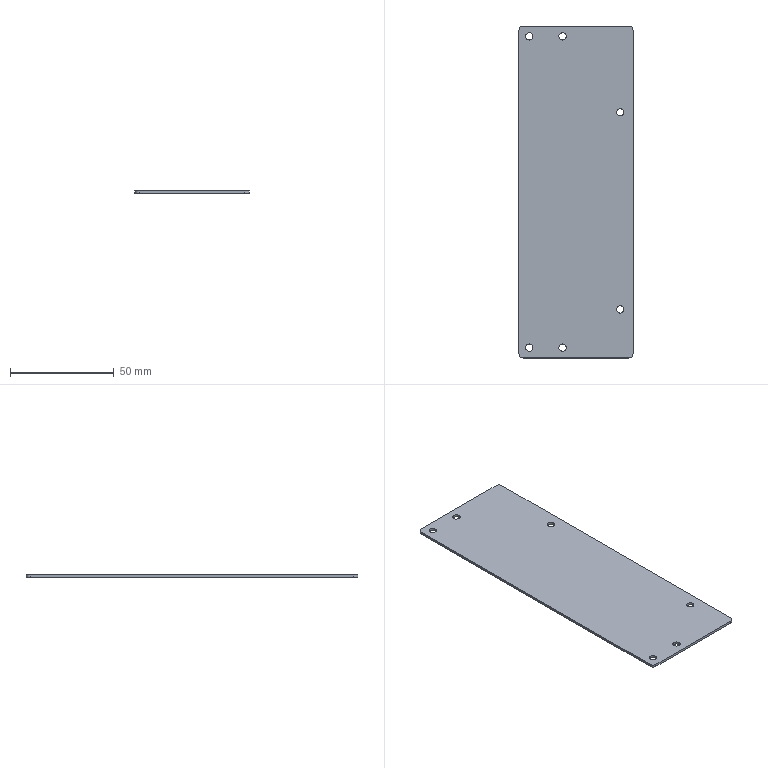Part | STEP file | Mounting block | 1 solid | 16 faces | box 55 x 160 x 1.2 mm | volume 10487 mm3 | cylinder 10 | plane 6 | commonest cylinder face diameters 3.5 x6 4 x4
STEP:
#1=CARTESIAN_POINT('',(0.,0.,0.));
#2=DIRECTION('',(0.,0.,1.));
#3=DIRECTION('',(1.,0.,0.));
#4=AXIS2_PLACEMENT_3D('',#1,#2,#3);
#5=CARTESIAN_POINT('',(-30.,-73.25,1.2));
#6=VERTEX_POINT('',#5);
#7=CARTESIAN_POINT('',(-28.25,-75.,1.2));
#8=VERTEX_POINT('',#7);
#9=CARTESIAN_POINT('',(-30.,-75.,1.2));
#10=DIRECTION('',(0.,0.,-1.));
#11=DIRECTION('',(0.,1.,0.));
#12=AXIS2_PLACEMENT_3D('',#9,#10,#11);
#13=CIRCLE('',#12,1.75);
#14=CARTESIAN_POINT('',(-33.,-78.,1.2));
#15=DIRECTION('',(0.,0.,1.));
#16=DIRECTION('',(1.,0.,0.));
#17=AXIS2_PLACEMENT_3D('',#14,#15,#16);
#18=PLANE('',#17);
#19=CARTESIAN_POINT('',(3.,4.75));
#20=CARTESIAN_POINT('',(6.031,4.75));
#21=CARTESIAN_POINT('',(4.516,2.125));
#22=CARTESIAN_POINT('',(3.,-0.5));
#23=CARTESIAN_POINT('',(1.484,2.125));
#24=CARTESIAN_POINT('',(-0.03109,4.75));
#25=CARTESIAN_POINT('',(3.,4.75));
#26=(BOUNDED_CURVE()B_SPLINE_CURVE(2,(#19,#20,#21,#22,#23,#24,#25),.UNSPECIFIED.,.T.,.F.)B_SPLINE_CURVE_WITH_KNOTS((1,2,2,2,2,1),(-2.094,0.,2.094,4.189,6.283,8.378),.UNSPECIFIED.)CURVE()GEOMETRIC_REPRESENTATION_ITEM()RATIONAL_B_SPLINE_CURVE((1.,0.5,1.,0.5,1.,0.5,1.))REPRESENTATION_ITEM(''));
#27=(GEOMETRIC_REPRESENTATION_CONTEXT(2)PARAMETRIC_REPRESENTATION_CONTEXT()REPRESENTATION_CONTEXT('',''));
#28=DEFINITIONAL_REPRESENTATION('',(#26),#27);
#29=PCURVE('',#18,#28);
#30=CARTESIAN_POINT('',(-30.,-75.,-0.3));
#31=DIRECTION('',(0.,0.,1.));
#32=DIRECTION('',(1.,0.,0.));
#33=AXIS2_PLACEMENT_3D('',#30,#31,#32);
#34=CYLINDRICAL_SURFACE('',#33,1.75);
#35=CARTESIAN_POINT('',(1.571,1.5));
#36=DIRECTION('',(-1.,0.));
#37=VECTOR('',#36,1.);
#38=LINE('',#35,#37);
#39=(GEOMETRIC_REPRESENTATION_CONTEXT(2)PARAMETRIC_REPRESENTATION_CONTEXT()REPRESENTATION_CONTEXT('',''));
#40=DEFINITIONAL_REPRESENTATION('',(#38),#39);
#41=PCURVE('',#34,#40);
#42=SURFACE_CURVE('',#13,(#29,#41),.PCURVE_S1.);
#43=EDGE_CURVE('',#6,#8,#42,.T.);
#44=ORIENTED_EDGE('',*,*,#43,.T.);
#45=CARTESIAN_POINT('',(-30.,-75.,1.2));
#46=DIRECTION('',(0.,0.,-1.));
#47=DIRECTION('',(0.,1.,0.));
#48=AXIS2_PLACEMENT_3D('',#45,#46,#47);
#49=CIRCLE('',#48,1.75);
#50=CARTESIAN_POINT('',(3.,4.75));
#51=CARTESIAN_POINT('',(6.031,4.75));
#52=CARTESIAN_POINT('',(4.516,2.125));
#53=CARTESIAN_POINT('',(3.,-0.5));
#54=CARTESIAN_POINT('',(1.484,2.125));
#55=CARTESIAN_POINT('',(-0.03109,4.75));
#56=CARTESIAN_POINT('',(3.,4.75));
#57=(BOUNDED_CURVE()B_SPLINE_CURVE(2,(#50,#51,#52,#53,#54,#55,#56),.UNSPECIFIED.,.T.,.F.)B_SPLINE_CURVE_WITH_KNOTS((1,2,2,2,2,1),(-2.094,0.,2.094,4.189,6.283,8.378),.UNSPECIFIED.)CURVE()GEOMETRIC_REPRESENTATION_ITEM()RATIONAL_B_SPLINE_CURVE((1.,0.5,1.,0.5,1.,0.5,1.))REPRESENTATION_ITEM(''));
#58=(GEOMETRIC_REPRESENTATION_CONTEXT(2)PARAMETRIC_REPRESENTATION_CONTEXT()REPRESENTATION_CONTEXT('',''));
#59=DEFINITIONAL_REPRESENTATION('',(#57),#58);
#60=PCURVE('',#18,#59);
#61=CARTESIAN_POINT('',(7.854,1.5));
#62=DIRECTION('',(-1.,0.));
#63=VECTOR('',#62,1.);
#64=LINE('',#61,#63);
#65=(GEOMETRIC_REPRESENTATION_CONTEXT(2)PARAMETRIC_REPRESENTATION_CONTEXT()REPRESENTATION_CONTEXT('',''));
#66=DEFINITIONAL_REPRESENTATION('',(#64),#65);
#67=PCURVE('',#34,#66);
#68=SURFACE_CURVE('',#49,(#60,#67),.PCURVE_S1.);
#69=EDGE_CURVE('',#8,#6,#68,.T.);
#70=ORIENTED_EDGE('',*,*,#69,.T.);
#71=EDGE_LOOP('',(#44,#70));
#72=FACE_BOUND('',#71,.T.);
#73=CARTESIAN_POINT('',(-14.,73.25,1.2));
#74=VERTEX_POINT('',#73);
#75=CARTESIAN_POINT('',(-12.25,75.,1.2));
#76=VERTEX_POINT('',#75);
#77=CARTESIAN_POINT('',(-14.,75.,1.2));
#78=DIRECTION('',(0.,0.,1.));
#79=DIRECTION('',(0.,-1.,0.));
#80=AXIS2_PLACEMENT_3D('',#77,#78,#79);
#81=CIRCLE('',#80,1.75);
#82=CARTESIAN_POINT('',(19.,153.));
#83=DIRECTION('',(0.,-1.));
#84=AXIS2_PLACEMENT_2D('',#82,#83);
#85=CIRCLE('',#84,1.75);
#86=(GEOMETRIC_REPRESENTATION_CONTEXT(2)PARAMETRIC_REPRESENTATION_CONTEXT()REPRESENTATION_CONTEXT('',''));
#87=DEFINITIONAL_REPRESENTATION('',(#85),#86);
#88=PCURVE('',#18,#87);
#89=CARTESIAN_POINT('',(-14.,75.,-0.3));
#90=DIRECTION('',(0.,0.,1.));
#91=DIRECTION('',(1.,0.,0.));
#92=AXIS2_PLACEMENT_3D('',#89,#90,#91);
#93=CYLINDRICAL_SURFACE('',#92,1.75);
#94=CARTESIAN_POINT('',(4.712,1.5));
#95=DIRECTION('',(1.,0.));
#96=VECTOR('',#95,1.);
#97=LINE('',#94,#96);
#98=(GEOMETRIC_REPRESENTATION_CONTEXT(2)PARAMETRIC_REPRESENTATION_CONTEXT()REPRESENTATION_CONTEXT('',''));
#99=DEFINITIONAL_REPRESENTATION('',(#97),#98);
#100=PCURVE('',#93,#99);
#101=SURFACE_CURVE('',#81,(#88,#100),.PCURVE_S1.);
#102=EDGE_CURVE('',#74,#76,#101,.T.);
#103=ORIENTED_EDGE('',*,*,#102,.F.);
#104=CARTESIAN_POINT('',(-14.,75.,1.2));
#105=DIRECTION('',(0.,0.,1.));
#106=DIRECTION('',(0.,-1.,0.));
#107=AXIS2_PLACEMENT_3D('',#104,#105,#106);
#108=CIRCLE('',#107,1.75);
#109=CARTESIAN_POINT('',(19.,153.));
#110=DIRECTION('',(0.,-1.));
#111=AXIS2_PLACEMENT_2D('',#109,#110);
#112=CIRCLE('',#111,1.75);
#113=(GEOMETRIC_REPRESENTATION_CONTEXT(2)PARAMETRIC_REPRESENTATION_CONTEXT()REPRESENTATION_CONTEXT('',''));
#114=DEFINITIONAL_REPRESENTATION('',(#112),#113);
#115=PCURVE('',#18,#114);
#116=CARTESIAN_POINT('',(-1.571,1.5));
#117=DIRECTION('',(1.,0.));
#118=VECTOR('',#117,1.);
#119=LINE('',#116,#118);
#120=(GEOMETRIC_REPRESENTATION_CONTEXT(2)PARAMETRIC_REPRESENTATION_CONTEXT()REPRESENTATION_CONTEXT('',''));
#121=DEFINITIONAL_REPRESENTATION('',(#119),#120);
#122=PCURVE('',#93,#121);
#123=SURFACE_CURVE('',#108,(#115,#122),.PCURVE_S1.);
#124=EDGE_CURVE('',#76,#74,#123,.T.);
#125=ORIENTED_EDGE('',*,*,#124,.F.);
#126=EDGE_LOOP('',(#103,#125));
#127=FACE_BOUND('',#126,.T.);
#128=CARTESIAN_POINT('',(15.595,-56.595,1.2));
#129=VERTEX_POINT('',#128);
#130=CARTESIAN_POINT('',(13.845,-54.845,1.2));
#131=VERTEX_POINT('',#130);
#132=CARTESIAN_POINT('',(13.845,-56.595,1.2));
#133=DIRECTION('',(0.,0.,1.));
#134=DIRECTION('',(1.,0.,0.));
#135=AXIS2_PLACEMENT_3D('',#132,#133,#134);
#136=CIRCLE('',#135,1.75);
#137=CARTESIAN_POINT('',(46.845,21.405));
#138=DIRECTION('',(1.,0.));
#139=AXIS2_PLACEMENT_2D('',#137,#138);
#140=CIRCLE('',#139,1.75);
#141=(GEOMETRIC_REPRESENTATION_CONTEXT(2)PARAMETRIC_REPRESENTATION_CONTEXT()REPRESENTATION_CONTEXT('',''));
#142=DEFINITIONAL_REPRESENTATION('',(#140),#141);
#143=PCURVE('',#18,#142);
#144=CARTESIAN_POINT('',(13.845,-56.595,1.5));
#145=DIRECTION('',(0.,0.,-1.));
#146=DIRECTION('',(-1.,0.,0.));
#147=AXIS2_PLACEMENT_3D('',#144,#145,#146);
#148=CYLINDRICAL_SURFACE('',#147,1.75);
#149=CARTESIAN_POINT('',(3.142,0.3));
#150=DIRECTION('',(-1.,0.));
#151=VECTOR('',#150,1.);
#152=LINE('',#149,#151);
#153=(GEOMETRIC_REPRESENTATION_CONTEXT(2)PARAMETRIC_REPRESENTATION_CONTEXT()REPRESENTATION_CONTEXT('',''));
#154=DEFINITIONAL_REPRESENTATION('',(#152),#153);
#155=PCURVE('',#148,#154);
#156=SURFACE_CURVE('',#136,(#143,#155),.PCURVE_S1.);
#157=EDGE_CURVE('',#129,#131,#156,.T.);
#158=ORIENTED_EDGE('',*,*,#157,.F.);
#159=CARTESIAN_POINT('',(13.845,-56.595,1.2));
#160=DIRECTION('',(0.,0.,1.));
#161=DIRECTION('',(1.,0.,0.));
#162=AXIS2_PLACEMENT_3D('',#159,#160,#161);
#163=CIRCLE('',#162,1.75);
#164=CARTESIAN_POINT('',(46.845,21.405));
#165=DIRECTION('',(1.,0.));
#166=AXIS2_PLACEMENT_2D('',#164,#165);
#167=CIRCLE('',#166,1.75);
#168=(GEOMETRIC_REPRESENTATION_CONTEXT(2)PARAMETRIC_REPRESENTATION_CONTEXT()REPRESENTATION_CONTEXT('',''));
#169=DEFINITIONAL_REPRESENTATION('',(#167),#168);
#170=PCURVE('',#18,#169);
#171=CARTESIAN_POINT('',(9.425,0.3));
#172=DIRECTION('',(-1.,0.));
#173=VECTOR('',#172,1.);
#174=LINE('',#171,#173);
#175=(GEOMETRIC_REPRESENTATION_CONTEXT(2)PARAMETRIC_REPRESENTATION_CONTEXT()REPRESENTATION_CONTEXT('',''));
#176=DEFINITIONAL_REPRESENTATION('',(#174),#175);
#177=PCURVE('',#148,#176);
#178=SURFACE_CURVE('',#163,(#170,#177),.PCURVE_S1.);
#179=EDGE_CURVE('',#131,#129,#178,.T.);
#180=ORIENTED_EDGE('',*,*,#179,.F.);
#181=EDGE_LOOP('',(#158,#180));
#182=FACE_BOUND('',#181,.T.);
#183=CARTESIAN_POINT('',(15.595,38.405,1.2));
#184=VERTEX_POINT('',#183);
#185=CARTESIAN_POINT('',(13.845,40.155,1.2));
#186=VERTEX_POINT('',#185);
#187=CARTESIAN_POINT('',(13.845,38.405,1.2));
#188=DIRECTION('',(0.,0.,1.));
#189=DIRECTION('',(1.,0.,0.));
#190=AXIS2_PLACEMENT_3D('',#187,#188,#189);
#191=CIRCLE('',#190,1.75);
#192=CARTESIAN_POINT('',(46.845,116.405));
#193=DIRECTION('',(1.,0.));
#194=AXIS2_PLACEMENT_2D('',#192,#193);
#195=CIRCLE('',#194,1.75);
#196=(GEOMETRIC_REPRESENTATION_CONTEXT(2)PARAMETRIC_REPRESENTATION_CONTEXT()REPRESENTATION_CONTEXT('',''));
#197=DEFINITIONAL_REPRESENTATION('',(#195),#196);
#198=PCURVE('',#18,#197);
#199=CARTESIAN_POINT('',(13.845,38.405,1.5));
#200=DIRECTION('',(0.,0.,-1.));
#201=DIRECTION('',(-1.,0.,0.));
#202=AXIS2_PLACEMENT_3D('',#199,#200,#201);
#203=CYLINDRICAL_SURFACE('',#202,1.75);
#204=CARTESIAN_POINT('',(3.142,0.3));
#205=DIRECTION('',(-1.,0.));
#206=VECTOR('',#205,1.);
#207=LINE('',#204,#206);
#208=(GEOMETRIC_REPRESENTATION_CONTEXT(2)PARAMETRIC_REPRESENTATION_CONTEXT()REPRESENTATION_CONTEXT('',''));
#209=DEFINITIONAL_REPRESENTATION('',(#207),#208);
#210=PCURVE('',#203,#209);
#211=SURFACE_CURVE('',#191,(#198,#210),.PCURVE_S1.);
#212=EDGE_CURVE('',#184,#186,#211,.T.);
#213=ORIENTED_EDGE('',*,*,#212,.F.);
#214=CARTESIAN_POINT('',(13.845,38.405,1.2));
#215=DIRECTION('',(0.,0.,1.));
#216=DIRECTION('',(1.,0.,0.));
#217=AXIS2_PLACEMENT_3D('',#214,#215,#216);
#218=CIRCLE('',#217,1.75);
#219=CARTESIAN_POINT('',(46.845,116.405));
#220=DIRECTION('',(1.,0.));
#221=AXIS2_PLACEMENT_2D('',#219,#220);
#222=CIRCLE('',#221,1.75);
#223=(GEOMETRIC_REPRESENTATION_CONTEXT(2)PARAMETRIC_REPRESENTATION_CONTEXT()REPRESENTATION_CONTEXT('',''));
#224=DEFINITIONAL_REPRESENTATION('',(#222),#223);
#225=PCURVE('',#18,#224);
#226=CARTESIAN_POINT('',(9.425,0.3));
#227=DIRECTION('',(-1.,0.));
#228=VECTOR('',#227,1.);
#229=LINE('',#226,#228);
#230=(GEOMETRIC_REPRESENTATION_CONTEXT(2)PARAMETRIC_REPRESENTATION_CONTEXT()REPRESENTATION_CONTEXT('',''));
#231=DEFINITIONAL_REPRESENTATION('',(#229),#230);
#232=PCURVE('',#203,#231);
#233=SURFACE_CURVE('',#218,(#225,#232),.PCURVE_S1.);
#234=EDGE_CURVE('',#186,#184,#233,.T.);
#235=ORIENTED_EDGE('',*,*,#234,.F.);
#236=EDGE_LOOP('',(#213,#235));
#237=FACE_BOUND('',#236,.T.);
#238=CARTESIAN_POINT('',(-35.,78.,1.2));
#239=VERTEX_POINT('',#238);
#240=CARTESIAN_POINT('',(-35.,-78.,1.2));
#241=VERTEX_POINT('',#240);
#242=CARTESIAN_POINT('',(-35.,78.,1.2));
#243=DIRECTION('',(0.,-1.,0.));
#244=VECTOR('',#243,1.);
#245=LINE('',#242,#244);
#246=CARTESIAN_POINT('',(-2.,156.));
#247=DIRECTION('',(0.,-1.));
#248=VECTOR('',#247,1.);
#249=LINE('',#246,#248);
#250=(GEOMETRIC_REPRESENTATION_CONTEXT(2)PARAMETRIC_REPRESENTATION_CONTEXT()REPRESENTATION_CONTEXT('',''));
#251=DEFINITIONAL_REPRESENTATION('',(#249),#250);
#252=PCURVE('',#18,#251);
#253=CARTESIAN_POINT('',(-35.,78.,1.2));
#254=DIRECTION('',(1.,0.,0.));
#255=DIRECTION('',(0.,1.,0.));
#256=AXIS2_PLACEMENT_3D('',#253,#254,#255);
#257=PLANE('',#256);
#258=CARTESIAN_POINT('',(0.,0.));
#259=DIRECTION('',(-1.,0.));
#260=VECTOR('',#259,1.);
#261=LINE('',#258,#260);
#262=(GEOMETRIC_REPRESENTATION_CONTEXT(2)PARAMETRIC_REPRESENTATION_CONTEXT()REPRESENTATION_CONTEXT('',''));
#263=DEFINITIONAL_REPRESENTATION('',(#261),#262);
#264=PCURVE('',#257,#263);
#265=SURFACE_CURVE('',#245,(#252,#264),.PCURVE_S1.);
#266=EDGE_CURVE('',#239,#241,#265,.T.);
#267=ORIENTED_EDGE('',*,*,#266,.T.);
#268=CARTESIAN_POINT('',(-33.,-80.,1.2));
#269=VERTEX_POINT('',#268);
#270=CARTESIAN_POINT('',(-33.,-78.,1.2));
#271=DIRECTION('',(0.,0.,1.));
#272=DIRECTION('',(1.,0.,0.));
#273=AXIS2_PLACEMENT_3D('',#270,#271,#272);
#274=CIRCLE('',#273,2.);
#275=CARTESIAN_POINT('',(0.,0.));
#276=DIRECTION('',(1.,0.));
#277=AXIS2_PLACEMENT_2D('',#275,#276);
#278=CIRCLE('',#277,2.);
#279=(GEOMETRIC_REPRESENTATION_CONTEXT(2)PARAMETRIC_REPRESENTATION_CONTEXT()REPRESENTATION_CONTEXT('',''));
#280=DEFINITIONAL_REPRESENTATION('',(#278),#279);
#281=PCURVE('',#18,#280);
#282=CARTESIAN_POINT('',(-33.,-78.,1.2));
#283=DIRECTION('',(0.,0.,-1.));
#284=DIRECTION('',(-1.,0.,0.));
#285=AXIS2_PLACEMENT_3D('',#282,#283,#284);
#286=CYLINDRICAL_SURFACE('',#285,2.);
#287=CARTESIAN_POINT('',(9.425,0.));
#288=DIRECTION('',(-1.,0.));
#289=VECTOR('',#288,1.);
#290=LINE('',#287,#289);
#291=(GEOMETRIC_REPRESENTATION_CONTEXT(2)PARAMETRIC_REPRESENTATION_CONTEXT()REPRESENTATION_CONTEXT('',''));
#292=DEFINITIONAL_REPRESENTATION('',(#290),#291);
#293=PCURVE('',#286,#292);
#294=SURFACE_CURVE('',#274,(#281,#293),.PCURVE_S1.);
#295=EDGE_CURVE('',#241,#269,#294,.T.);
#296=ORIENTED_EDGE('',*,*,#295,.T.);
#297=CARTESIAN_POINT('',(18.,-80.,1.2));
#298=VERTEX_POINT('',#297);
#299=CARTESIAN_POINT('',(-33.,-80.,1.2));
#300=DIRECTION('',(1.,0.,0.));
#301=VECTOR('',#300,1.);
#302=LINE('',#299,#301);
#303=CARTESIAN_POINT('',(0.,-2.));
#304=DIRECTION('',(1.,0.));
#305=VECTOR('',#304,1.);
#306=LINE('',#303,#305);
#307=(GEOMETRIC_REPRESENTATION_CONTEXT(2)PARAMETRIC_REPRESENTATION_CONTEXT()REPRESENTATION_CONTEXT('',''));
#308=DEFINITIONAL_REPRESENTATION('',(#306),#307);
#309=PCURVE('',#18,#308);
#310=CARTESIAN_POINT('',(-33.,-80.,1.2));
#311=DIRECTION('',(0.,1.,0.));
#312=DIRECTION('',(0.,0.,1.));
#313=AXIS2_PLACEMENT_3D('',#310,#311,#312);
#314=PLANE('',#313);
#315=CARTESIAN_POINT('',(0.,0.));
#316=DIRECTION('',(0.,1.));
#317=VECTOR('',#316,1.);
#318=LINE('',#315,#317);
#319=(GEOMETRIC_REPRESENTATION_CONTEXT(2)PARAMETRIC_REPRESENTATION_CONTEXT()REPRESENTATION_CONTEXT('',''));
#320=DEFINITIONAL_REPRESENTATION('',(#318),#319);
#321=PCURVE('',#314,#320);
#322=SURFACE_CURVE('',#302,(#309,#321),.PCURVE_S1.);
#323=EDGE_CURVE('',#269,#298,#322,.T.);
#324=ORIENTED_EDGE('',*,*,#323,.T.);
#325=CARTESIAN_POINT('',(20.,-78.,1.2));
#326=VERTEX_POINT('',#325);
#327=CARTESIAN_POINT('',(18.,-78.,1.2));
#328=DIRECTION('',(0.,0.,1.));
#329=DIRECTION('',(1.,0.,0.));
#330=AXIS2_PLACEMENT_3D('',#327,#328,#329);
#331=CIRCLE('',#330,2.);
#332=CARTESIAN_POINT('',(51.,0.));
#333=DIRECTION('',(1.,0.));
#334=AXIS2_PLACEMENT_2D('',#332,#333);
#335=CIRCLE('',#334,2.);
#336=(GEOMETRIC_REPRESENTATION_CONTEXT(2)PARAMETRIC_REPRESENTATION_CONTEXT()REPRESENTATION_CONTEXT('',''));
#337=DEFINITIONAL_REPRESENTATION('',(#335),#336);
#338=PCURVE('',#18,#337);
#339=CARTESIAN_POINT('',(18.,-78.,1.2));
#340=DIRECTION('',(0.,0.,-1.));
#341=DIRECTION('',(-1.,0.,0.));
#342=AXIS2_PLACEMENT_3D('',#339,#340,#341);
#343=CYLINDRICAL_SURFACE('',#342,2.);
#344=CARTESIAN_POINT('',(9.425,0.));
#345=DIRECTION('',(-1.,0.));
#346=VECTOR('',#345,1.);
#347=LINE('',#344,#346);
#348=(GEOMETRIC_REPRESENTATION_CONTEXT(2)PARAMETRIC_REPRESENTATION_CONTEXT()REPRESENTATION_CONTEXT('',''));
#349=DEFINITIONAL_REPRESENTATION('',(#347),#348);
#350=PCURVE('',#343,#349);
#351=SURFACE_CURVE('',#331,(#338,#350),.PCURVE_S1.);
#352=EDGE_CURVE('',#298,#326,#351,.T.);
#353=ORIENTED_EDGE('',*,*,#352,.T.);
#354=CARTESIAN_POINT('',(20.,78.,1.2));
#355=VERTEX_POINT('',#354);
#356=CARTESIAN_POINT('',(20.,-78.,1.2));
#357=DIRECTION('',(0.,1.,0.));
#358=VECTOR('',#357,1.);
#359=LINE('',#356,#358);
#360=CARTESIAN_POINT('',(53.,0.));
#361=DIRECTION('',(0.,1.));
#362=VECTOR('',#361,1.);
#363=LINE('',#360,#362);
#364=(GEOMETRIC_REPRESENTATION_CONTEXT(2)PARAMETRIC_REPRESENTATION_CONTEXT()REPRESENTATION_CONTEXT('',''));
#365=DEFINITIONAL_REPRESENTATION('',(#363),#364);
#366=PCURVE('',#18,#365);
#367=CARTESIAN_POINT('',(20.,-78.,1.2));
#368=DIRECTION('',(-1.,0.,0.));
#369=DIRECTION('',(0.,-1.,0.));
#370=AXIS2_PLACEMENT_3D('',#367,#368,#369);
#371=PLANE('',#370);
#372=CARTESIAN_POINT('',(0.,0.));
#373=DIRECTION('',(-1.,0.));
#374=VECTOR('',#373,1.);
#375=LINE('',#372,#374);
#376=(GEOMETRIC_REPRESENTATION_CONTEXT(2)PARAMETRIC_REPRESENTATION_CONTEXT()REPRESENTATION_CONTEXT('',''));
#377=DEFINITIONAL_REPRESENTATION('',(#375),#376);
#378=PCURVE('',#371,#377);
#379=SURFACE_CURVE('',#359,(#366,#378),.PCURVE_S1.);
#380=EDGE_CURVE('',#326,#355,#379,.T.);
#381=ORIENTED_EDGE('',*,*,#380,.T.);
#382=CARTESIAN_POINT('',(18.,80.,1.2));
#383=VERTEX_POINT('',#382);
#384=CARTESIAN_POINT('',(18.,78.,1.2));
#385=DIRECTION('',(0.,0.,1.));
#386=DIRECTION('',(1.,0.,0.));
#387=AXIS2_PLACEMENT_3D('',#384,#385,#386);
#388=CIRCLE('',#387,2.);
#389=CARTESIAN_POINT('',(51.,156.));
#390=DIRECTION('',(1.,0.));
#391=AXIS2_PLACEMENT_2D('',#389,#390);
#392=CIRCLE('',#391,2.);
#393=(GEOMETRIC_REPRESENTATION_CONTEXT(2)PARAMETRIC_REPRESENTATION_CONTEXT()REPRESENTATION_CONTEXT('',''));
#394=DEFINITIONAL_REPRESENTATION('',(#392),#393);
#395=PCURVE('',#18,#394);
#396=CARTESIAN_POINT('',(18.,78.,1.2));
#397=DIRECTION('',(0.,0.,-1.));
#398=DIRECTION('',(-1.,0.,0.));
#399=AXIS2_PLACEMENT_3D('',#396,#397,#398);
#400=CYLINDRICAL_SURFACE('',#399,2.);
#401=CARTESIAN_POINT('',(3.142,0.));
#402=DIRECTION('',(-1.,0.));
#403=VECTOR('',#402,1.);
#404=LINE('',#401,#403);
#405=(GEOMETRIC_REPRESENTATION_CONTEXT(2)PARAMETRIC_REPRESENTATION_CONTEXT()REPRESENTATION_CONTEXT('',''));
#406=DEFINITIONAL_REPRESENTATION('',(#404),#405);
#407=PCURVE('',#400,#406);
#408=SURFACE_CURVE('',#388,(#395,#407),.PCURVE_S1.);
#409=EDGE_CURVE('',#355,#383,#408,.T.);
#410=ORIENTED_EDGE('',*,*,#409,.T.);
#411=CARTESIAN_POINT('',(-33.,80.,1.2));
#412=VERTEX_POINT('',#411);
#413=CARTESIAN_POINT('',(18.,80.,1.2));
#414=DIRECTION('',(-1.,0.,0.));
#415=VECTOR('',#414,1.);
#416=LINE('',#413,#415);
#417=CARTESIAN_POINT('',(51.,158.));
#418=DIRECTION('',(-1.,0.));
#419=VECTOR('',#418,1.);
#420=LINE('',#417,#419);
#421=(GEOMETRIC_REPRESENTATION_CONTEXT(2)PARAMETRIC_REPRESENTATION_CONTEXT()REPRESENTATION_CONTEXT('',''));
#422=DEFINITIONAL_REPRESENTATION('',(#420),#421);
#423=PCURVE('',#18,#422);
#424=CARTESIAN_POINT('',(18.,80.,1.2));
#425=DIRECTION('',(0.,-1.,0.));
#426=DIRECTION('',(0.,0.,-1.));
#427=AXIS2_PLACEMENT_3D('',#424,#425,#426);
#428=PLANE('',#427);
#429=CARTESIAN_POINT('',(0.,0.));
#430=DIRECTION('',(0.,-1.));
#431=VECTOR('',#430,1.);
#432=LINE('',#429,#431);
#433=(GEOMETRIC_REPRESENTATION_CONTEXT(2)PARAMETRIC_REPRESENTATION_CONTEXT()REPRESENTATION_CONTEXT('',''));
#434=DEFINITIONAL_REPRESENTATION('',(#432),#433);
#435=PCURVE('',#428,#434);
#436=SURFACE_CURVE('',#416,(#423,#435),.PCURVE_S1.);
#437=EDGE_CURVE('',#383,#412,#436,.T.);
#438=ORIENTED_EDGE('',*,*,#437,.T.);
#439=CARTESIAN_POINT('',(-33.,78.,1.2));
#440=DIRECTION('',(0.,0.,1.));
#441=DIRECTION('',(1.,0.,0.));
#442=AXIS2_PLACEMENT_3D('',#439,#440,#441);
#443=CIRCLE('',#442,2.);
#444=CARTESIAN_POINT('',(0.,156.));
#445=DIRECTION('',(1.,0.));
#446=AXIS2_PLACEMENT_2D('',#444,#445);
#447=CIRCLE('',#446,2.);
#448=(GEOMETRIC_REPRESENTATION_CONTEXT(2)PARAMETRIC_REPRESENTATION_CONTEXT()REPRESENTATION_CONTEXT('',''));
#449=DEFINITIONAL_REPRESENTATION('',(#447),#448);
#450=PCURVE('',#18,#449);
#451=CARTESIAN_POINT('',(-33.,78.,1.2));
#452=DIRECTION('',(0.,0.,-1.));
#453=DIRECTION('',(-1.,0.,0.));
#454=AXIS2_PLACEMENT_3D('',#451,#452,#453);
#455=CYLINDRICAL_SURFACE('',#454,2.);
#456=CARTESIAN_POINT('',(3.142,0.));
#457=DIRECTION('',(-1.,0.));
#458=VECTOR('',#457,1.);
#459=LINE('',#456,#458);
#460=(GEOMETRIC_REPRESENTATION_CONTEXT(2)PARAMETRIC_REPRESENTATION_CONTEXT()REPRESENTATION_CONTEXT('',''));
#461=DEFINITIONAL_REPRESENTATION('',(#459),#460);
#462=PCURVE('',#455,#461);
#463=SURFACE_CURVE('',#443,(#450,#462),.PCURVE_S1.);
#464=EDGE_CURVE('',#412,#239,#463,.T.);
#465=ORIENTED_EDGE('',*,*,#464,.T.);
#466=EDGE_LOOP('',(#267,#296,#324,#353,#381,#410,#438,#465));
#467=FACE_BOUND('',#466,.T.);
#468=CARTESIAN_POINT('',(-30.,73.25,1.2));
#469=VERTEX_POINT('',#468);
#470=CARTESIAN_POINT('',(-28.25,75.,1.2));
#471=VERTEX_POINT('',#470);
#472=CARTESIAN_POINT('',(-30.,75.,1.2));
#473=DIRECTION('',(0.,0.,1.));
#474=DIRECTION('',(0.,-1.,0.));
#475=AXIS2_PLACEMENT_3D('',#472,#473,#474);
#476=CIRCLE('',#475,1.75);
#477=CARTESIAN_POINT('',(3.,153.));
#478=DIRECTION('',(0.,-1.));
#479=AXIS2_PLACEMENT_2D('',#477,#478);
#480=CIRCLE('',#479,1.75);
#481=(GEOMETRIC_REPRESENTATION_CONTEXT(2)PARAMETRIC_REPRESENTATION_CONTEXT()REPRESENTATION_CONTEXT('',''));
#482=DEFINITIONAL_REPRESENTATION('',(#480),#481);
#483=PCURVE('',#18,#482);
#484=CARTESIAN_POINT('',(-30.,75.,-0.3));
#485=DIRECTION('',(0.,0.,1.));
#486=DIRECTION('',(1.,0.,0.));
#487=AXIS2_PLACEMENT_3D('',#484,#485,#486);
#488=CYLINDRICAL_SURFACE('',#487,1.75);
#489=CARTESIAN_POINT('',(4.712,1.5));
#490=DIRECTION('',(1.,0.));
#491=VECTOR('',#490,1.);
#492=LINE('',#489,#491);
#493=(GEOMETRIC_REPRESENTATION_CONTEXT(2)PARAMETRIC_REPRESENTATION_CONTEXT()REPRESENTATION_CONTEXT('',''));
#494=DEFINITIONAL_REPRESENTATION('',(#492),#493);
#495=PCURVE('',#488,#494);
#496=SURFACE_CURVE('',#476,(#483,#495),.PCURVE_S1.);
#497=EDGE_CURVE('',#469,#471,#496,.T.);
#498=ORIENTED_EDGE('',*,*,#497,.F.);
#499=CARTESIAN_POINT('',(-30.,75.,1.2));
#500=DIRECTION('',(0.,0.,1.));
#501=DIRECTION('',(0.,-1.,0.));
#502=AXIS2_PLACEMENT_3D('',#499,#500,#501);
#503=CIRCLE('',#502,1.75);
#504=CARTESIAN_POINT('',(3.,153.));
#505=DIRECTION('',(0.,-1.));
#506=AXIS2_PLACEMENT_2D('',#504,#505);
#507=CIRCLE('',#506,1.75);
#508=(GEOMETRIC_REPRESENTATION_CONTEXT(2)PARAMETRIC_REPRESENTATION_CONTEXT()REPRESENTATION_CONTEXT('',''));
#509=DEFINITIONAL_REPRESENTATION('',(#507),#508);
#510=PCURVE('',#18,#509);
#511=CARTESIAN_POINT('',(-1.571,1.5));
#512=DIRECTION('',(1.,0.));
#513=VECTOR('',#512,1.);
#514=LINE('',#511,#513);
#515=(GEOMETRIC_REPRESENTATION_CONTEXT(2)PARAMETRIC_REPRESENTATION_CONTEXT()REPRESENTATION_CONTEXT('',''));
#516=DEFINITIONAL_REPRESENTATION('',(#514),#515);
#517=PCURVE('',#488,#516);
#518=SURFACE_CURVE('',#503,(#510,#517),.PCURVE_S1.);
#519=EDGE_CURVE('',#471,#469,#518,.T.);
#520=ORIENTED_EDGE('',*,*,#519,.F.);
#521=EDGE_LOOP('',(#498,#520));
#522=FACE_BOUND('',#521,.T.);
#523=CARTESIAN_POINT('',(-14.,-73.25,1.2));
#524=VERTEX_POINT('',#523);
#525=CARTESIAN_POINT('',(-12.25,-75.,1.2));
#526=VERTEX_POINT('',#525);
#527=CARTESIAN_POINT('',(-14.,-75.,1.2));
#528=DIRECTION('',(0.,0.,-1.));
#529=DIRECTION('',(0.,1.,0.));
#530=AXIS2_PLACEMENT_3D('',#527,#528,#529);
#531=CIRCLE('',#530,1.75);
#532=CARTESIAN_POINT('',(19.,4.75));
#533=CARTESIAN_POINT('',(22.031,4.75));
#534=CARTESIAN_POINT('',(20.516,2.125));
#535=CARTESIAN_POINT('',(19.,-0.5));
#536=CARTESIAN_POINT('',(17.484,2.125));
#537=CARTESIAN_POINT('',(15.969,4.75));
#538=CARTESIAN_POINT('',(19.,4.75));
#539=(BOUNDED_CURVE()B_SPLINE_CURVE(2,(#532,#533,#534,#535,#536,#537,#538),.UNSPECIFIED.,.T.,.F.)B_SPLINE_CURVE_WITH_KNOTS((1,2,2,2,2,1),(-2.094,0.,2.094,4.189,6.283,8.378),.UNSPECIFIED.)CURVE()GEOMETRIC_REPRESENTATION_ITEM()RATIONAL_B_SPLINE_CURVE((1.,0.5,1.,0.5,1.,0.5,1.))REPRESENTATION_ITEM(''));
#540=(GEOMETRIC_REPRESENTATION_CONTEXT(2)PARAMETRIC_REPRESENTATION_CONTEXT()REPRESENTATION_CONTEXT('',''));
#541=DEFINITIONAL_REPRESENTATION('',(#539),#540);
#542=PCURVE('',#18,#541);
#543=CARTESIAN_POINT('',(-14.,-75.,-0.3));
#544=DIRECTION('',(0.,0.,1.));
#545=DIRECTION('',(1.,0.,0.));
#546=AXIS2_PLACEMENT_3D('',#543,#544,#545);
#547=CYLINDRICAL_SURFACE('',#546,1.75);
#548=CARTESIAN_POINT('',(1.571,1.5));
#549=DIRECTION('',(-1.,0.));
#550=VECTOR('',#549,1.);
#551=LINE('',#548,#550);
#552=(GEOMETRIC_REPRESENTATION_CONTEXT(2)PARAMETRIC_REPRESENTATION_CONTEXT()REPRESENTATION_CONTEXT('',''));
#553=DEFINITIONAL_REPRESENTATION('',(#551),#552);
#554=PCURVE('',#547,#553);
#555=SURFACE_CURVE('',#531,(#542,#554),.PCURVE_S1.);
#556=EDGE_CURVE('',#524,#526,#555,.T.);
#557=ORIENTED_EDGE('',*,*,#556,.T.);
#558=CARTESIAN_POINT('',(-14.,-75.,1.2));
#559=DIRECTION('',(0.,0.,-1.));
#560=DIRECTION('',(0.,1.,0.));
#561=AXIS2_PLACEMENT_3D('',#558,#559,#560);
#562=CIRCLE('',#561,1.75);
#563=CARTESIAN_POINT('',(19.,4.75));
#564=CARTESIAN_POINT('',(22.031,4.75));
#565=CARTESIAN_POINT('',(20.516,2.125));
#566=CARTESIAN_POINT('',(19.,-0.5));
#567=CARTESIAN_POINT('',(17.484,2.125));
#568=CARTESIAN_POINT('',(15.969,4.75));
#569=CARTESIAN_POINT('',(19.,4.75));
#570=(BOUNDED_CURVE()B_SPLINE_CURVE(2,(#563,#564,#565,#566,#567,#568,#569),.UNSPECIFIED.,.T.,.F.)B_SPLINE_CURVE_WITH_KNOTS((1,2,2,2,2,1),(-2.094,0.,2.094,4.189,6.283,8.378),.UNSPECIFIED.)CURVE()GEOMETRIC_REPRESENTATION_ITEM()RATIONAL_B_SPLINE_CURVE((1.,0.5,1.,0.5,1.,0.5,1.))REPRESENTATION_ITEM(''));
#571=(GEOMETRIC_REPRESENTATION_CONTEXT(2)PARAMETRIC_REPRESENTATION_CONTEXT()REPRESENTATION_CONTEXT('',''));
#572=DEFINITIONAL_REPRESENTATION('',(#570),#571);
#573=PCURVE('',#18,#572);
#574=CARTESIAN_POINT('',(7.854,1.5));
#575=DIRECTION('',(-1.,0.));
#576=VECTOR('',#575,1.);
#577=LINE('',#574,#576);
#578=(GEOMETRIC_REPRESENTATION_CONTEXT(2)PARAMETRIC_REPRESENTATION_CONTEXT()REPRESENTATION_CONTEXT('',''));
#579=DEFINITIONAL_REPRESENTATION('',(#577),#578);
#580=PCURVE('',#547,#579);
#581=SURFACE_CURVE('',#562,(#573,#580),.PCURVE_S1.);
#582=EDGE_CURVE('',#526,#524,#581,.T.);
#583=ORIENTED_EDGE('',*,*,#582,.T.);
#584=EDGE_LOOP('',(#557,#583));
#585=FACE_BOUND('',#584,.T.);
#586=ADVANCED_FACE('',(#72,#127,#182,#237,#467,#522,#585),#18,.T.);
#587=CARTESIAN_POINT('',(-28.25,75.,0.));
#588=VERTEX_POINT('',#587);
#589=CARTESIAN_POINT('',(-30.,75.,0.));
#590=DIRECTION('',(0.,0.,1.));
#591=DIRECTION('',(1.,0.,0.));
#592=AXIS2_PLACEMENT_3D('',#589,#590,#591);
#593=CIRCLE('',#592,1.75);
#594=CARTESIAN_POINT('',(-33.,-78.,0.));
#595=DIRECTION('',(0.,0.,1.));
#596=DIRECTION('',(1.,0.,0.));
#597=AXIS2_PLACEMENT_3D('',#594,#595,#596);
#598=PLANE('',#597);
#599=CARTESIAN_POINT('',(3.,153.));
#600=DIRECTION('',(1.,0.));
#601=AXIS2_PLACEMENT_2D('',#599,#600);
#602=CIRCLE('',#601,1.75);
#603=(GEOMETRIC_REPRESENTATION_CONTEXT(2)PARAMETRIC_REPRESENTATION_CONTEXT()REPRESENTATION_CONTEXT('',''));
#604=DEFINITIONAL_REPRESENTATION('',(#602),#603);
#605=PCURVE('',#598,#604);
#606=CARTESIAN_POINT('',(0.,0.3));
#607=DIRECTION('',(1.,0.));
#608=VECTOR('',#607,1.);
#609=LINE('',#606,#608);
#610=(GEOMETRIC_REPRESENTATION_CONTEXT(2)PARAMETRIC_REPRESENTATION_CONTEXT()REPRESENTATION_CONTEXT('',''));
#611=DEFINITIONAL_REPRESENTATION('',(#609),#610);
#612=PCURVE('',#488,#611);
#613=SURFACE_CURVE('',#593,(#605,#612),.PCURVE_S1.);
#614=EDGE_CURVE('',#588,#588,#613,.T.);
#615=ORIENTED_EDGE('',*,*,#614,.T.);
#616=EDGE_LOOP('',(#615));
#617=FACE_BOUND('',#616,.T.);
#618=CARTESIAN_POINT('',(-12.25,75.,0.));
#619=VERTEX_POINT('',#618);
#620=CARTESIAN_POINT('',(-14.,75.,0.));
#621=DIRECTION('',(0.,0.,1.));
#622=DIRECTION('',(1.,0.,0.));
#623=AXIS2_PLACEMENT_3D('',#620,#621,#622);
#624=CIRCLE('',#623,1.75);
#625=CARTESIAN_POINT('',(19.,153.));
#626=DIRECTION('',(1.,0.));
#627=AXIS2_PLACEMENT_2D('',#625,#626);
#628=CIRCLE('',#627,1.75);
#629=(GEOMETRIC_REPRESENTATION_CONTEXT(2)PARAMETRIC_REPRESENTATION_CONTEXT()REPRESENTATION_CONTEXT('',''));
#630=DEFINITIONAL_REPRESENTATION('',(#628),#629);
#631=PCURVE('',#598,#630);
#632=CARTESIAN_POINT('',(0.,0.3));
#633=DIRECTION('',(1.,0.));
#634=VECTOR('',#633,1.);
#635=LINE('',#632,#634);
#636=(GEOMETRIC_REPRESENTATION_CONTEXT(2)PARAMETRIC_REPRESENTATION_CONTEXT()REPRESENTATION_CONTEXT('',''));
#637=DEFINITIONAL_REPRESENTATION('',(#635),#636);
#638=PCURVE('',#93,#637);
#639=SURFACE_CURVE('',#624,(#631,#638),.PCURVE_S1.);
#640=EDGE_CURVE('',#619,#619,#639,.T.);
#641=ORIENTED_EDGE('',*,*,#640,.T.);
#642=EDGE_LOOP('',(#641));
#643=FACE_BOUND('',#642,.T.);
#644=CARTESIAN_POINT('',(13.845,-54.845,0.));
#645=VERTEX_POINT('',#644);
#646=CARTESIAN_POINT('',(13.845,-56.595,0.));
#647=DIRECTION('',(0.,0.,-1.));
#648=DIRECTION('',(0.,1.,0.));
#649=AXIS2_PLACEMENT_3D('',#646,#647,#648);
#650=CIRCLE('',#649,1.75);
#651=CARTESIAN_POINT('',(46.845,23.155));
#652=CARTESIAN_POINT('',(49.876,23.155));
#653=CARTESIAN_POINT('',(48.361,20.53));
#654=CARTESIAN_POINT('',(46.845,17.905));
#655=CARTESIAN_POINT('',(45.33,20.53));
#656=CARTESIAN_POINT('',(43.814,23.155));
#657=CARTESIAN_POINT('',(46.845,23.155));
#658=(BOUNDED_CURVE()B_SPLINE_CURVE(2,(#651,#652,#653,#654,#655,#656,#657),.UNSPECIFIED.,.T.,.F.)B_SPLINE_CURVE_WITH_KNOTS((1,2,2,2,2,1),(-2.094,0.,2.094,4.189,6.283,8.378),.UNSPECIFIED.)CURVE()GEOMETRIC_REPRESENTATION_ITEM()RATIONAL_B_SPLINE_CURVE((1.,0.5,1.,0.5,1.,0.5,1.))REPRESENTATION_ITEM(''));
#659=(GEOMETRIC_REPRESENTATION_CONTEXT(2)PARAMETRIC_REPRESENTATION_CONTEXT()REPRESENTATION_CONTEXT('',''));
#660=DEFINITIONAL_REPRESENTATION('',(#658),#659);
#661=PCURVE('',#598,#660);
#662=CARTESIAN_POINT('',(1.571,1.5));
#663=DIRECTION('',(1.,0.));
#664=VECTOR('',#663,1.);
#665=LINE('',#662,#664);
#666=(GEOMETRIC_REPRESENTATION_CONTEXT(2)PARAMETRIC_REPRESENTATION_CONTEXT()REPRESENTATION_CONTEXT('',''));
#667=DEFINITIONAL_REPRESENTATION('',(#665),#666);
#668=PCURVE('',#148,#667);
#669=SURFACE_CURVE('',#650,(#661,#668),.PCURVE_S1.);
#670=EDGE_CURVE('',#645,#645,#669,.T.);
#671=ORIENTED_EDGE('',*,*,#670,.F.);
#672=EDGE_LOOP('',(#671));
#673=FACE_BOUND('',#672,.T.);
#674=CARTESIAN_POINT('',(13.845,40.155,0.));
#675=VERTEX_POINT('',#674);
#676=CARTESIAN_POINT('',(13.845,38.405,0.));
#677=DIRECTION('',(0.,0.,-1.));
#678=DIRECTION('',(0.,1.,0.));
#679=AXIS2_PLACEMENT_3D('',#676,#677,#678);
#680=CIRCLE('',#679,1.75);
#681=CARTESIAN_POINT('',(46.845,118.155));
#682=CARTESIAN_POINT('',(49.876,118.155));
#683=CARTESIAN_POINT('',(48.361,115.53));
#684=CARTESIAN_POINT('',(46.845,112.905));
#685=CARTESIAN_POINT('',(45.33,115.53));
#686=CARTESIAN_POINT('',(43.814,118.155));
#687=CARTESIAN_POINT('',(46.845,118.155));
#688=(BOUNDED_CURVE()B_SPLINE_CURVE(2,(#681,#682,#683,#684,#685,#686,#687),.UNSPECIFIED.,.T.,.F.)B_SPLINE_CURVE_WITH_KNOTS((1,2,2,2,2,1),(-2.094,0.,2.094,4.189,6.283,8.378),.UNSPECIFIED.)CURVE()GEOMETRIC_REPRESENTATION_ITEM()RATIONAL_B_SPLINE_CURVE((1.,0.5,1.,0.5,1.,0.5,1.))REPRESENTATION_ITEM(''));
#689=(GEOMETRIC_REPRESENTATION_CONTEXT(2)PARAMETRIC_REPRESENTATION_CONTEXT()REPRESENTATION_CONTEXT('',''));
#690=DEFINITIONAL_REPRESENTATION('',(#688),#689);
#691=PCURVE('',#598,#690);
#692=CARTESIAN_POINT('',(1.571,1.5));
#693=DIRECTION('',(1.,0.));
#694=VECTOR('',#693,1.);
#695=LINE('',#692,#694);
#696=(GEOMETRIC_REPRESENTATION_CONTEXT(2)PARAMETRIC_REPRESENTATION_CONTEXT()REPRESENTATION_CONTEXT('',''));
#697=DEFINITIONAL_REPRESENTATION('',(#695),#696);
#698=PCURVE('',#203,#697);
#699=SURFACE_CURVE('',#680,(#691,#698),.PCURVE_S1.);
#700=EDGE_CURVE('',#675,#675,#699,.T.);
#701=ORIENTED_EDGE('',*,*,#700,.F.);
#702=EDGE_LOOP('',(#701));
#703=FACE_BOUND('',#702,.T.);
#704=CARTESIAN_POINT('',(-35.,78.,0.));
#705=VERTEX_POINT('',#704);
#706=CARTESIAN_POINT('',(-35.,-78.,0.));
#707=VERTEX_POINT('',#706);
#708=CARTESIAN_POINT('',(-35.,78.,0.));
#709=DIRECTION('',(0.,-1.,0.));
#710=VECTOR('',#709,1.);
#711=LINE('',#708,#710);
#712=CARTESIAN_POINT('',(-2.,156.));
#713=DIRECTION('',(0.,-1.));
#714=VECTOR('',#713,1.);
#715=LINE('',#712,#714);
#716=(GEOMETRIC_REPRESENTATION_CONTEXT(2)PARAMETRIC_REPRESENTATION_CONTEXT()REPRESENTATION_CONTEXT('',''));
#717=DEFINITIONAL_REPRESENTATION('',(#715),#716);
#718=PCURVE('',#598,#717);
#719=CARTESIAN_POINT('',(0.,-1.2));
#720=DIRECTION('',(-1.,0.));
#721=VECTOR('',#720,1.);
#722=LINE('',#719,#721);
#723=(GEOMETRIC_REPRESENTATION_CONTEXT(2)PARAMETRIC_REPRESENTATION_CONTEXT()REPRESENTATION_CONTEXT('',''));
#724=DEFINITIONAL_REPRESENTATION('',(#722),#723);
#725=PCURVE('',#257,#724);
#726=SURFACE_CURVE('',#711,(#718,#725),.PCURVE_S1.);
#727=EDGE_CURVE('',#705,#707,#726,.T.);
#728=ORIENTED_EDGE('',*,*,#727,.F.);
#729=CARTESIAN_POINT('',(-33.,80.,0.));
#730=VERTEX_POINT('',#729);
#731=CARTESIAN_POINT('',(-33.,78.,0.));
#732=DIRECTION('',(0.,0.,1.));
#733=DIRECTION('',(1.,0.,0.));
#734=AXIS2_PLACEMENT_3D('',#731,#732,#733);
#735=CIRCLE('',#734,2.);
#736=CARTESIAN_POINT('',(0.,156.));
#737=DIRECTION('',(1.,0.));
#738=AXIS2_PLACEMENT_2D('',#736,#737);
#739=CIRCLE('',#738,2.);
#740=(GEOMETRIC_REPRESENTATION_CONTEXT(2)PARAMETRIC_REPRESENTATION_CONTEXT()REPRESENTATION_CONTEXT('',''));
#741=DEFINITIONAL_REPRESENTATION('',(#739),#740);
#742=PCURVE('',#598,#741);
#743=CARTESIAN_POINT('',(3.142,1.2));
#744=DIRECTION('',(-1.,0.));
#745=VECTOR('',#744,1.);
#746=LINE('',#743,#745);
#747=(GEOMETRIC_REPRESENTATION_CONTEXT(2)PARAMETRIC_REPRESENTATION_CONTEXT()REPRESENTATION_CONTEXT('',''));
#748=DEFINITIONAL_REPRESENTATION('',(#746),#747);
#749=PCURVE('',#455,#748);
#750=SURFACE_CURVE('',#735,(#742,#749),.PCURVE_S1.);
#751=EDGE_CURVE('',#730,#705,#750,.T.);
#752=ORIENTED_EDGE('',*,*,#751,.F.);
#753=CARTESIAN_POINT('',(18.,80.,0.));
#754=VERTEX_POINT('',#753);
#755=CARTESIAN_POINT('',(18.,80.,0.));
#756=DIRECTION('',(-1.,0.,0.));
#757=VECTOR('',#756,1.);
#758=LINE('',#755,#757);
#759=CARTESIAN_POINT('',(51.,158.));
#760=DIRECTION('',(-1.,0.));
#761=VECTOR('',#760,1.);
#762=LINE('',#759,#761);
#763=(GEOMETRIC_REPRESENTATION_CONTEXT(2)PARAMETRIC_REPRESENTATION_CONTEXT()REPRESENTATION_CONTEXT('',''));
#764=DEFINITIONAL_REPRESENTATION('',(#762),#763);
#765=PCURVE('',#598,#764);
#766=CARTESIAN_POINT('',(1.2,0.));
#767=DIRECTION('',(0.,-1.));
#768=VECTOR('',#767,1.);
#769=LINE('',#766,#768);
#770=(GEOMETRIC_REPRESENTATION_CONTEXT(2)PARAMETRIC_REPRESENTATION_CONTEXT()REPRESENTATION_CONTEXT('',''));
#771=DEFINITIONAL_REPRESENTATION('',(#769),#770);
#772=PCURVE('',#428,#771);
#773=SURFACE_CURVE('',#758,(#765,#772),.PCURVE_S1.);
#774=EDGE_CURVE('',#754,#730,#773,.T.);
#775=ORIENTED_EDGE('',*,*,#774,.F.);
#776=CARTESIAN_POINT('',(20.,78.,0.));
#777=VERTEX_POINT('',#776);
#778=CARTESIAN_POINT('',(18.,78.,0.));
#779=DIRECTION('',(0.,0.,1.));
#780=DIRECTION('',(1.,0.,0.));
#781=AXIS2_PLACEMENT_3D('',#778,#779,#780);
#782=CIRCLE('',#781,2.);
#783=CARTESIAN_POINT('',(51.,156.));
#784=DIRECTION('',(1.,0.));
#785=AXIS2_PLACEMENT_2D('',#783,#784);
#786=CIRCLE('',#785,2.);
#787=(GEOMETRIC_REPRESENTATION_CONTEXT(2)PARAMETRIC_REPRESENTATION_CONTEXT()REPRESENTATION_CONTEXT('',''));
#788=DEFINITIONAL_REPRESENTATION('',(#786),#787);
#789=PCURVE('',#598,#788);
#790=CARTESIAN_POINT('',(3.142,1.2));
#791=DIRECTION('',(-1.,0.));
#792=VECTOR('',#791,1.);
#793=LINE('',#790,#792);
#794=(GEOMETRIC_REPRESENTATION_CONTEXT(2)PARAMETRIC_REPRESENTATION_CONTEXT()REPRESENTATION_CONTEXT('',''));
#795=DEFINITIONAL_REPRESENTATION('',(#793),#794);
#796=PCURVE('',#400,#795);
#797=SURFACE_CURVE('',#782,(#789,#796),.PCURVE_S1.);
#798=EDGE_CURVE('',#777,#754,#797,.T.);
#799=ORIENTED_EDGE('',*,*,#798,.F.);
#800=CARTESIAN_POINT('',(20.,-78.,0.));
#801=VERTEX_POINT('',#800);
#802=CARTESIAN_POINT('',(20.,-78.,0.));
#803=DIRECTION('',(0.,1.,0.));
#804=VECTOR('',#803,1.);
#805=LINE('',#802,#804);
#806=CARTESIAN_POINT('',(53.,0.));
#807=DIRECTION('',(0.,1.));
#808=VECTOR('',#807,1.);
#809=LINE('',#806,#808);
#810=(GEOMETRIC_REPRESENTATION_CONTEXT(2)PARAMETRIC_REPRESENTATION_CONTEXT()REPRESENTATION_CONTEXT('',''));
#811=DEFINITIONAL_REPRESENTATION('',(#809),#810);
#812=PCURVE('',#598,#811);
#813=CARTESIAN_POINT('',(0.,-1.2));
#814=DIRECTION('',(-1.,0.));
#815=VECTOR('',#814,1.);
#816=LINE('',#813,#815);
#817=(GEOMETRIC_REPRESENTATION_CONTEXT(2)PARAMETRIC_REPRESENTATION_CONTEXT()REPRESENTATION_CONTEXT('',''));
#818=DEFINITIONAL_REPRESENTATION('',(#816),#817);
#819=PCURVE('',#371,#818);
#820=SURFACE_CURVE('',#805,(#812,#819),.PCURVE_S1.);
#821=EDGE_CURVE('',#801,#777,#820,.T.);
#822=ORIENTED_EDGE('',*,*,#821,.F.);
#823=CARTESIAN_POINT('',(18.,-80.,0.));
#824=VERTEX_POINT('',#823);
#825=CARTESIAN_POINT('',(18.,-78.,0.));
#826=DIRECTION('',(0.,0.,1.));
#827=DIRECTION('',(1.,0.,0.));
#828=AXIS2_PLACEMENT_3D('',#825,#826,#827);
#829=CIRCLE('',#828,2.);
#830=CARTESIAN_POINT('',(51.,0.));
#831=DIRECTION('',(1.,0.));
#832=AXIS2_PLACEMENT_2D('',#830,#831);
#833=CIRCLE('',#832,2.);
#834=(GEOMETRIC_REPRESENTATION_CONTEXT(2)PARAMETRIC_REPRESENTATION_CONTEXT()REPRESENTATION_CONTEXT('',''));
#835=DEFINITIONAL_REPRESENTATION('',(#833),#834);
#836=PCURVE('',#598,#835);
#837=CARTESIAN_POINT('',(9.425,1.2));
#838=DIRECTION('',(-1.,0.));
#839=VECTOR('',#838,1.);
#840=LINE('',#837,#839);
#841=(GEOMETRIC_REPRESENTATION_CONTEXT(2)PARAMETRIC_REPRESENTATION_CONTEXT()REPRESENTATION_CONTEXT('',''));
#842=DEFINITIONAL_REPRESENTATION('',(#840),#841);
#843=PCURVE('',#343,#842);
#844=SURFACE_CURVE('',#829,(#836,#843),.PCURVE_S1.);
#845=EDGE_CURVE('',#824,#801,#844,.T.);
#846=ORIENTED_EDGE('',*,*,#845,.F.);
#847=CARTESIAN_POINT('',(-33.,-80.,0.));
#848=VERTEX_POINT('',#847);
#849=CARTESIAN_POINT('',(-33.,-80.,0.));
#850=DIRECTION('',(1.,0.,0.));
#851=VECTOR('',#850,1.);
#852=LINE('',#849,#851);
#853=CARTESIAN_POINT('',(0.,-2.));
#854=DIRECTION('',(1.,0.));
#855=VECTOR('',#854,1.);
#856=LINE('',#853,#855);
#857=(GEOMETRIC_REPRESENTATION_CONTEXT(2)PARAMETRIC_REPRESENTATION_CONTEXT()REPRESENTATION_CONTEXT('',''));
#858=DEFINITIONAL_REPRESENTATION('',(#856),#857);
#859=PCURVE('',#598,#858);
#860=CARTESIAN_POINT('',(-1.2,0.));
#861=DIRECTION('',(0.,1.));
#862=VECTOR('',#861,1.);
#863=LINE('',#860,#862);
#864=(GEOMETRIC_REPRESENTATION_CONTEXT(2)PARAMETRIC_REPRESENTATION_CONTEXT()REPRESENTATION_CONTEXT('',''));
#865=DEFINITIONAL_REPRESENTATION('',(#863),#864);
#866=PCURVE('',#314,#865);
#867=SURFACE_CURVE('',#852,(#859,#866),.PCURVE_S1.);
#868=EDGE_CURVE('',#848,#824,#867,.T.);
#869=ORIENTED_EDGE('',*,*,#868,.F.);
#870=CARTESIAN_POINT('',(-33.,-78.,0.));
#871=DIRECTION('',(0.,0.,1.));
#872=DIRECTION('',(1.,0.,0.));
#873=AXIS2_PLACEMENT_3D('',#870,#871,#872);
#874=CIRCLE('',#873,2.);
#875=CARTESIAN_POINT('',(0.,0.));
#876=DIRECTION('',(1.,0.));
#877=AXIS2_PLACEMENT_2D('',#875,#876);
#878=CIRCLE('',#877,2.);
#879=(GEOMETRIC_REPRESENTATION_CONTEXT(2)PARAMETRIC_REPRESENTATION_CONTEXT()REPRESENTATION_CONTEXT('',''));
#880=DEFINITIONAL_REPRESENTATION('',(#878),#879);
#881=PCURVE('',#598,#880);
#882=CARTESIAN_POINT('',(9.425,1.2));
#883=DIRECTION('',(-1.,0.));
#884=VECTOR('',#883,1.);
#885=LINE('',#882,#884);
#886=(GEOMETRIC_REPRESENTATION_CONTEXT(2)PARAMETRIC_REPRESENTATION_CONTEXT()REPRESENTATION_CONTEXT('',''));
#887=DEFINITIONAL_REPRESENTATION('',(#885),#886);
#888=PCURVE('',#286,#887);
#889=SURFACE_CURVE('',#874,(#881,#888),.PCURVE_S1.);
#890=EDGE_CURVE('',#707,#848,#889,.T.);
#891=ORIENTED_EDGE('',*,*,#890,.F.);
#892=EDGE_LOOP('',(#728,#752,#775,#799,#822,#846,#869,#891));
#893=FACE_BOUND('',#892,.T.);
#894=CARTESIAN_POINT('',(-28.25,-75.,0.));
#895=VERTEX_POINT('',#894);
#896=CARTESIAN_POINT('',(-30.,-75.,0.));
#897=DIRECTION('',(0.,0.,-1.));
#898=DIRECTION('',(1.,0.,0.));
#899=AXIS2_PLACEMENT_3D('',#896,#897,#898);
#900=CIRCLE('',#899,1.75);
#901=CARTESIAN_POINT('',(4.75,3.));
#902=CARTESIAN_POINT('',(4.75,-0.03109));
#903=CARTESIAN_POINT('',(2.125,1.484));
#904=CARTESIAN_POINT('',(-0.5,3.));
#905=CARTESIAN_POINT('',(2.125,4.516));
#906=CARTESIAN_POINT('',(4.75,6.031));
#907=CARTESIAN_POINT('',(4.75,3.));
#908=(BOUNDED_CURVE()B_SPLINE_CURVE(2,(#901,#902,#903,#904,#905,#906,#907),.UNSPECIFIED.,.T.,.F.)B_SPLINE_CURVE_WITH_KNOTS((1,2,2,2,2,1),(-2.094,0.,2.094,4.189,6.283,8.378),.UNSPECIFIED.)CURVE()GEOMETRIC_REPRESENTATION_ITEM()RATIONAL_B_SPLINE_CURVE((1.,0.5,1.,0.5,1.,0.5,1.))REPRESENTATION_ITEM(''));
#909=(GEOMETRIC_REPRESENTATION_CONTEXT(2)PARAMETRIC_REPRESENTATION_CONTEXT()REPRESENTATION_CONTEXT('',''));
#910=DEFINITIONAL_REPRESENTATION('',(#908),#909);
#911=PCURVE('',#598,#910);
#912=CARTESIAN_POINT('',(6.283,0.3));
#913=DIRECTION('',(-1.,0.));
#914=VECTOR('',#913,1.);
#915=LINE('',#912,#914);
#916=(GEOMETRIC_REPRESENTATION_CONTEXT(2)PARAMETRIC_REPRESENTATION_CONTEXT()REPRESENTATION_CONTEXT('',''));
#917=DEFINITIONAL_REPRESENTATION('',(#915),#916);
#918=PCURVE('',#34,#917);
#919=SURFACE_CURVE('',#900,(#911,#918),.PCURVE_S1.);
#920=EDGE_CURVE('',#895,#895,#919,.T.);
#921=ORIENTED_EDGE('',*,*,#920,.F.);
#922=EDGE_LOOP('',(#921));
#923=FACE_BOUND('',#922,.T.);
#924=CARTESIAN_POINT('',(-12.25,-75.,0.));
#925=VERTEX_POINT('',#924);
#926=CARTESIAN_POINT('',(-14.,-75.,0.));
#927=DIRECTION('',(0.,0.,-1.));
#928=DIRECTION('',(1.,0.,0.));
#929=AXIS2_PLACEMENT_3D('',#926,#927,#928);
#930=CIRCLE('',#929,1.75);
#931=CARTESIAN_POINT('',(20.75,3.));
#932=CARTESIAN_POINT('',(20.75,-0.03109));
#933=CARTESIAN_POINT('',(18.125,1.484));
#934=CARTESIAN_POINT('',(15.5,3.));
#935=CARTESIAN_POINT('',(18.125,4.516));
#936=CARTESIAN_POINT('',(20.75,6.031));
#937=CARTESIAN_POINT('',(20.75,3.));
#938=(BOUNDED_CURVE()B_SPLINE_CURVE(2,(#931,#932,#933,#934,#935,#936,#937),.UNSPECIFIED.,.T.,.F.)B_SPLINE_CURVE_WITH_KNOTS((1,2,2,2,2,1),(-2.094,0.,2.094,4.189,6.283,8.378),.UNSPECIFIED.)CURVE()GEOMETRIC_REPRESENTATION_ITEM()RATIONAL_B_SPLINE_CURVE((1.,0.5,1.,0.5,1.,0.5,1.))REPRESENTATION_ITEM(''));
#939=(GEOMETRIC_REPRESENTATION_CONTEXT(2)PARAMETRIC_REPRESENTATION_CONTEXT()REPRESENTATION_CONTEXT('',''));
#940=DEFINITIONAL_REPRESENTATION('',(#938),#939);
#941=PCURVE('',#598,#940);
#942=CARTESIAN_POINT('',(6.283,0.3));
#943=DIRECTION('',(-1.,0.));
#944=VECTOR('',#943,1.);
#945=LINE('',#942,#944);
#946=(GEOMETRIC_REPRESENTATION_CONTEXT(2)PARAMETRIC_REPRESENTATION_CONTEXT()REPRESENTATION_CONTEXT('',''));
#947=DEFINITIONAL_REPRESENTATION('',(#945),#946);
#948=PCURVE('',#547,#947);
#949=SURFACE_CURVE('',#930,(#941,#948),.PCURVE_S1.);
#950=EDGE_CURVE('',#925,#925,#949,.T.);
#951=ORIENTED_EDGE('',*,*,#950,.F.);
#952=EDGE_LOOP('',(#951));
#953=FACE_BOUND('',#952,.T.);
#954=ADVANCED_FACE('',(#617,#643,#673,#703,#893,#923,#953),#598,.F.);
#955=ORIENTED_EDGE('',*,*,#727,.T.);
#956=CARTESIAN_POINT('',(-35.,-78.,1.2));
#957=DIRECTION('',(0.,0.,-1.));
#958=VECTOR('',#957,1.);
#959=LINE('',#956,#958);
#960=CARTESIAN_POINT('',(-156.,0.));
#961=DIRECTION('',(0.,-1.));
#962=VECTOR('',#961,1.);
#963=LINE('',#960,#962);
#964=(GEOMETRIC_REPRESENTATION_CONTEXT(2)PARAMETRIC_REPRESENTATION_CONTEXT()REPRESENTATION_CONTEXT('',''));
#965=DEFINITIONAL_REPRESENTATION('',(#963),#964);
#966=PCURVE('',#257,#965);
#967=CARTESIAN_POINT('',(6.283,0.));
#968=DIRECTION('',(0.,1.));
#969=VECTOR('',#968,1.);
#970=LINE('',#967,#969);
#971=(GEOMETRIC_REPRESENTATION_CONTEXT(2)PARAMETRIC_REPRESENTATION_CONTEXT()REPRESENTATION_CONTEXT('',''));
#972=DEFINITIONAL_REPRESENTATION('',(#970),#971);
#973=PCURVE('',#286,#972);
#974=SURFACE_CURVE('',#959,(#966,#973),.PCURVE_S1.);
#975=EDGE_CURVE('',#241,#707,#974,.T.);
#976=ORIENTED_EDGE('',*,*,#975,.F.);
#977=ORIENTED_EDGE('',*,*,#266,.F.);
#978=CARTESIAN_POINT('',(-35.,78.,1.2));
#979=DIRECTION('',(0.,0.,-1.));
#980=VECTOR('',#979,1.);
#981=LINE('',#978,#980);
#982=CARTESIAN_POINT('',(0.,0.));
#983=DIRECTION('',(0.,-1.));
#984=VECTOR('',#983,1.);
#985=LINE('',#982,#984);
#986=(GEOMETRIC_REPRESENTATION_CONTEXT(2)PARAMETRIC_REPRESENTATION_CONTEXT()REPRESENTATION_CONTEXT('',''));
#987=DEFINITIONAL_REPRESENTATION('',(#985),#986);
#988=PCURVE('',#257,#987);
#989=CARTESIAN_POINT('',(0.,0.));
#990=DIRECTION('',(0.,1.));
#991=VECTOR('',#990,1.);
#992=LINE('',#989,#991);
#993=(GEOMETRIC_REPRESENTATION_CONTEXT(2)PARAMETRIC_REPRESENTATION_CONTEXT()REPRESENTATION_CONTEXT('',''));
#994=DEFINITIONAL_REPRESENTATION('',(#992),#993);
#995=PCURVE('',#455,#994);
#996=SURFACE_CURVE('',#981,(#988,#995),.PCURVE_S1.);
#997=EDGE_CURVE('',#239,#705,#996,.T.);
#998=ORIENTED_EDGE('',*,*,#997,.T.);
#999=EDGE_LOOP('',(#955,#976,#977,#998));
#1000=FACE_BOUND('',#999,.T.);
#1001=ADVANCED_FACE('',(#1000),#257,.F.);
#1002=ORIENTED_EDGE('',*,*,#890,.T.);
#1003=CARTESIAN_POINT('',(-33.,-80.,1.2));
#1004=DIRECTION('',(0.,0.,-1.));
#1005=VECTOR('',#1004,1.);
#1006=LINE('',#1003,#1005);
#1007=CARTESIAN_POINT('',(4.712,0.));
#1008=DIRECTION('',(0.,1.));
#1009=VECTOR('',#1008,1.);
#1010=LINE('',#1007,#1009);
#1011=(GEOMETRIC_REPRESENTATION_CONTEXT(2)PARAMETRIC_REPRESENTATION_CONTEXT()REPRESENTATION_CONTEXT('',''));
#1012=DEFINITIONAL_REPRESENTATION('',(#1010),#1011);
#1013=PCURVE('',#286,#1012);
#1014=CARTESIAN_POINT('',(0.,0.));
#1015=DIRECTION('',(-1.,0.));
#1016=VECTOR('',#1015,1.);
#1017=LINE('',#1014,#1016);
#1018=(GEOMETRIC_REPRESENTATION_CONTEXT(2)PARAMETRIC_REPRESENTATION_CONTEXT()REPRESENTATION_CONTEXT('',''));
#1019=DEFINITIONAL_REPRESENTATION('',(#1017),#1018);
#1020=PCURVE('',#314,#1019);
#1021=SURFACE_CURVE('',#1006,(#1013,#1020),.PCURVE_S1.);
#1022=EDGE_CURVE('',#269,#848,#1021,.T.);
#1023=ORIENTED_EDGE('',*,*,#1022,.F.);
#1024=ORIENTED_EDGE('',*,*,#295,.F.);
#1025=ORIENTED_EDGE('',*,*,#975,.T.);
#1026=EDGE_LOOP('',(#1002,#1023,#1024,#1025));
#1027=FACE_BOUND('',#1026,.T.);
#1028=ADVANCED_FACE('',(#1027),#286,.T.);
#1029=ORIENTED_EDGE('',*,*,#868,.T.);
#1030=CARTESIAN_POINT('',(18.,-80.,1.2));
#1031=DIRECTION('',(0.,0.,-1.));
#1032=VECTOR('',#1031,1.);
#1033=LINE('',#1030,#1032);
#1034=CARTESIAN_POINT('',(0.,51.));
#1035=DIRECTION('',(-1.,0.));
#1036=VECTOR('',#1035,1.);
#1037=LINE('',#1034,#1036);
#1038=(GEOMETRIC_REPRESENTATION_CONTEXT(2)PARAMETRIC_REPRESENTATION_CONTEXT()REPRESENTATION_CONTEXT('',''));
#1039=DEFINITIONAL_REPRESENTATION('',(#1037),#1038);
#1040=PCURVE('',#314,#1039);
#1041=CARTESIAN_POINT('',(4.712,0.));
#1042=DIRECTION('',(0.,1.));
#1043=VECTOR('',#1042,1.);
#1044=LINE('',#1041,#1043);
#1045=(GEOMETRIC_REPRESENTATION_CONTEXT(2)PARAMETRIC_REPRESENTATION_CONTEXT()REPRESENTATION_CONTEXT('',''));
#1046=DEFINITIONAL_REPRESENTATION('',(#1044),#1045);
#1047=PCURVE('',#343,#1046);
#1048=SURFACE_CURVE('',#1033,(#1040,#1047),.PCURVE_S1.);
#1049=EDGE_CURVE('',#298,#824,#1048,.T.);
#1050=ORIENTED_EDGE('',*,*,#1049,.F.);
#1051=ORIENTED_EDGE('',*,*,#323,.F.);
#1052=ORIENTED_EDGE('',*,*,#1022,.T.);
#1053=EDGE_LOOP('',(#1029,#1050,#1051,#1052));
#1054=FACE_BOUND('',#1053,.T.);
#1055=ADVANCED_FACE('',(#1054),#314,.F.);
#1056=ORIENTED_EDGE('',*,*,#845,.T.);
#1057=CARTESIAN_POINT('',(20.,-78.,1.2));
#1058=DIRECTION('',(0.,0.,-1.));
#1059=VECTOR('',#1058,1.);
#1060=LINE('',#1057,#1059);
#1061=CARTESIAN_POINT('',(3.142,0.));
#1062=DIRECTION('',(0.,1.));
#1063=VECTOR('',#1062,1.);
#1064=LINE('',#1061,#1063);
#1065=(GEOMETRIC_REPRESENTATION_CONTEXT(2)PARAMETRIC_REPRESENTATION_CONTEXT()REPRESENTATION_CONTEXT('',''));
#1066=DEFINITIONAL_REPRESENTATION('',(#1064),#1065);
#1067=PCURVE('',#343,#1066);
#1068=CARTESIAN_POINT('',(0.,0.));
#1069=DIRECTION('',(0.,-1.));
#1070=VECTOR('',#1069,1.);
#1071=LINE('',#1068,#1070);
#1072=(GEOMETRIC_REPRESENTATION_CONTEXT(2)PARAMETRIC_REPRESENTATION_CONTEXT()REPRESENTATION_CONTEXT('',''));
#1073=DEFINITIONAL_REPRESENTATION('',(#1071),#1072);
#1074=PCURVE('',#371,#1073);
#1075=SURFACE_CURVE('',#1060,(#1067,#1074),.PCURVE_S1.);
#1076=EDGE_CURVE('',#326,#801,#1075,.T.);
#1077=ORIENTED_EDGE('',*,*,#1076,.F.);
#1078=ORIENTED_EDGE('',*,*,#352,.F.);
#1079=ORIENTED_EDGE('',*,*,#1049,.T.);
#1080=EDGE_LOOP('',(#1056,#1077,#1078,#1079));
#1081=FACE_BOUND('',#1080,.T.);
#1082=ADVANCED_FACE('',(#1081),#343,.T.);
#1083=ORIENTED_EDGE('',*,*,#821,.T.);
#1084=CARTESIAN_POINT('',(20.,78.,1.2));
#1085=DIRECTION('',(0.,0.,-1.));
#1086=VECTOR('',#1085,1.);
#1087=LINE('',#1084,#1086);
#1088=CARTESIAN_POINT('',(-156.,0.));
#1089=DIRECTION('',(0.,-1.));
#1090=VECTOR('',#1089,1.);
#1091=LINE('',#1088,#1090);
#1092=(GEOMETRIC_REPRESENTATION_CONTEXT(2)PARAMETRIC_REPRESENTATION_CONTEXT()REPRESENTATION_CONTEXT('',''));
#1093=DEFINITIONAL_REPRESENTATION('',(#1091),#1092);
#1094=PCURVE('',#371,#1093);
#1095=CARTESIAN_POINT('',(3.142,0.));
#1096=DIRECTION('',(0.,1.));
#1097=VECTOR('',#1096,1.);
#1098=LINE('',#1095,#1097);
#1099=(GEOMETRIC_REPRESENTATION_CONTEXT(2)PARAMETRIC_REPRESENTATION_CONTEXT()REPRESENTATION_CONTEXT('',''));
#1100=DEFINITIONAL_REPRESENTATION('',(#1098),#1099);
#1101=PCURVE('',#400,#1100);
#1102=SURFACE_CURVE('',#1087,(#1094,#1101),.PCURVE_S1.);
#1103=EDGE_CURVE('',#355,#777,#1102,.T.);
#1104=ORIENTED_EDGE('',*,*,#1103,.F.);
#1105=ORIENTED_EDGE('',*,*,#380,.F.);
#1106=ORIENTED_EDGE('',*,*,#1076,.T.);
#1107=EDGE_LOOP('',(#1083,#1104,#1105,#1106));
#1108=FACE_BOUND('',#1107,.T.);
#1109=ADVANCED_FACE('',(#1108),#371,.F.);
#1110=ORIENTED_EDGE('',*,*,#798,.T.);
#1111=CARTESIAN_POINT('',(18.,80.,1.2));
#1112=DIRECTION('',(0.,0.,-1.));
#1113=VECTOR('',#1112,1.);
#1114=LINE('',#1111,#1113);
#1115=CARTESIAN_POINT('',(1.571,0.));
#1116=DIRECTION('',(0.,1.));
#1117=VECTOR('',#1116,1.);
#1118=LINE('',#1115,#1117);
#1119=(GEOMETRIC_REPRESENTATION_CONTEXT(2)PARAMETRIC_REPRESENTATION_CONTEXT()REPRESENTATION_CONTEXT('',''));
#1120=DEFINITIONAL_REPRESENTATION('',(#1118),#1119);
#1121=PCURVE('',#400,#1120);
#1122=CARTESIAN_POINT('',(0.,0.));
#1123=DIRECTION('',(1.,0.));
#1124=VECTOR('',#1123,1.);
#1125=LINE('',#1122,#1124);
#1126=(GEOMETRIC_REPRESENTATION_CONTEXT(2)PARAMETRIC_REPRESENTATION_CONTEXT()REPRESENTATION_CONTEXT('',''));
#1127=DEFINITIONAL_REPRESENTATION('',(#1125),#1126);
#1128=PCURVE('',#428,#1127);
#1129=SURFACE_CURVE('',#1114,(#1121,#1128),.PCURVE_S1.);
#1130=EDGE_CURVE('',#383,#754,#1129,.T.);
#1131=ORIENTED_EDGE('',*,*,#1130,.F.);
#1132=ORIENTED_EDGE('',*,*,#409,.F.);
#1133=ORIENTED_EDGE('',*,*,#1103,.T.);
#1134=EDGE_LOOP('',(#1110,#1131,#1132,#1133));
#1135=FACE_BOUND('',#1134,.T.);
#1136=ADVANCED_FACE('',(#1135),#400,.T.);
#1137=ORIENTED_EDGE('',*,*,#774,.T.);
#1138=CARTESIAN_POINT('',(-33.,80.,1.2));
#1139=DIRECTION('',(0.,0.,-1.));
#1140=VECTOR('',#1139,1.);
#1141=LINE('',#1138,#1140);
#1142=CARTESIAN_POINT('',(0.,-51.));
#1143=DIRECTION('',(1.,0.));
#1144=VECTOR('',#1143,1.);
#1145=LINE('',#1142,#1144);
#1146=(GEOMETRIC_REPRESENTATION_CONTEXT(2)PARAMETRIC_REPRESENTATION_CONTEXT()REPRESENTATION_CONTEXT('',''));
#1147=DEFINITIONAL_REPRESENTATION('',(#1145),#1146);
#1148=PCURVE('',#428,#1147);
#1149=CARTESIAN_POINT('',(1.571,0.));
#1150=DIRECTION('',(0.,1.));
#1151=VECTOR('',#1150,1.);
#1152=LINE('',#1149,#1151);
#1153=(GEOMETRIC_REPRESENTATION_CONTEXT(2)PARAMETRIC_REPRESENTATION_CONTEXT()REPRESENTATION_CONTEXT('',''));
#1154=DEFINITIONAL_REPRESENTATION('',(#1152),#1153);
#1155=PCURVE('',#455,#1154);
#1156=SURFACE_CURVE('',#1141,(#1148,#1155),.PCURVE_S1.);
#1157=EDGE_CURVE('',#412,#730,#1156,.T.);
#1158=ORIENTED_EDGE('',*,*,#1157,.F.);
#1159=ORIENTED_EDGE('',*,*,#437,.F.);
#1160=ORIENTED_EDGE('',*,*,#1130,.T.);
#1161=EDGE_LOOP('',(#1137,#1158,#1159,#1160));
#1162=FACE_BOUND('',#1161,.T.);
#1163=ADVANCED_FACE('',(#1162),#428,.F.);
#1164=ORIENTED_EDGE('',*,*,#751,.T.);
#1165=ORIENTED_EDGE('',*,*,#997,.F.);
#1166=ORIENTED_EDGE('',*,*,#464,.F.);
#1167=ORIENTED_EDGE('',*,*,#1157,.T.);
#1168=EDGE_LOOP('',(#1164,#1165,#1166,#1167));
#1169=FACE_BOUND('',#1168,.T.);
#1170=ADVANCED_FACE('',(#1169),#455,.T.);
#1171=ORIENTED_EDGE('',*,*,#234,.F.);
#1172=CARTESIAN_POINT('',(13.845,40.155,1.2));
#1173=CARTESIAN_POINT('',(13.845,40.155,0.));
#1174=B_SPLINE_CURVE_WITH_KNOTS('',1,(#1172,#1173),.UNSPECIFIED.,.F.,.F.,(2,2),(0.3,1.5),.PIECEWISE_BEZIER_KNOTS.);
#1175=CARTESIAN_POINT('',(7.854,0.));
#1176=DIRECTION('',(0.,1.));
#1177=VECTOR('',#1176,1.);
#1178=LINE('',#1175,#1177);
#1179=(GEOMETRIC_REPRESENTATION_CONTEXT(2)PARAMETRIC_REPRESENTATION_CONTEXT()REPRESENTATION_CONTEXT('',''));
#1180=DEFINITIONAL_REPRESENTATION('',(#1178),#1179);
#1181=PCURVE('',#203,#1180);
#1182=CARTESIAN_POINT('',(1.571,0.));
#1183=DIRECTION('',(0.,1.));
#1184=VECTOR('',#1183,1.);
#1185=LINE('',#1182,#1184);
#1186=(GEOMETRIC_REPRESENTATION_CONTEXT(2)PARAMETRIC_REPRESENTATION_CONTEXT()REPRESENTATION_CONTEXT('',''));
#1187=DEFINITIONAL_REPRESENTATION('',(#1185),#1186);
#1188=PCURVE('',#203,#1187);
#1189=SEAM_CURVE('',#1174,(#1181,#1188),.PCURVE_S1.);
#1190=EDGE_CURVE('',#186,#675,#1189,.T.);
#1191=ORIENTED_EDGE('',*,*,#1190,.T.);
#1192=ORIENTED_EDGE('',*,*,#700,.F.);
#1193=ORIENTED_EDGE('',*,*,#1190,.F.);
#1194=ORIENTED_EDGE('',*,*,#212,.F.);
#1195=EDGE_LOOP('',(#1171,#1191,#1192,#1193,#1194));
#1196=FACE_BOUND('',#1195,.F.);
#1197=ADVANCED_FACE('',(#1196),#203,.F.);
#1198=ORIENTED_EDGE('',*,*,#179,.F.);
#1199=CARTESIAN_POINT('',(13.845,-54.845,1.2));
#1200=CARTESIAN_POINT('',(13.845,-54.845,0.));
#1201=B_SPLINE_CURVE_WITH_KNOTS('',1,(#1199,#1200),.UNSPECIFIED.,.F.,.F.,(2,2),(0.3,1.5),.PIECEWISE_BEZIER_KNOTS.);
#1202=CARTESIAN_POINT('',(7.854,0.));
#1203=DIRECTION('',(0.,1.));
#1204=VECTOR('',#1203,1.);
#1205=LINE('',#1202,#1204);
#1206=(GEOMETRIC_REPRESENTATION_CONTEXT(2)PARAMETRIC_REPRESENTATION_CONTEXT()REPRESENTATION_CONTEXT('',''));
#1207=DEFINITIONAL_REPRESENTATION('',(#1205),#1206);
#1208=PCURVE('',#148,#1207);
#1209=CARTESIAN_POINT('',(1.571,0.));
#1210=DIRECTION('',(0.,1.));
#1211=VECTOR('',#1210,1.);
#1212=LINE('',#1209,#1211);
#1213=(GEOMETRIC_REPRESENTATION_CONTEXT(2)PARAMETRIC_REPRESENTATION_CONTEXT()REPRESENTATION_CONTEXT('',''));
#1214=DEFINITIONAL_REPRESENTATION('',(#1212),#1213);
#1215=PCURVE('',#148,#1214);
#1216=SEAM_CURVE('',#1201,(#1208,#1215),.PCURVE_S1.);
#1217=EDGE_CURVE('',#131,#645,#1216,.T.);
#1218=ORIENTED_EDGE('',*,*,#1217,.T.);
#1219=ORIENTED_EDGE('',*,*,#670,.F.);
#1220=ORIENTED_EDGE('',*,*,#1217,.F.);
#1221=ORIENTED_EDGE('',*,*,#157,.F.);
#1222=EDGE_LOOP('',(#1198,#1218,#1219,#1220,#1221));
#1223=FACE_BOUND('',#1222,.F.);
#1224=ADVANCED_FACE('',(#1223),#148,.F.);
#1225=ORIENTED_EDGE('',*,*,#124,.F.);
#1226=CARTESIAN_POINT('',(-12.25,75.,0.));
#1227=CARTESIAN_POINT('',(-12.25,75.,1.2));
#1228=B_SPLINE_CURVE_WITH_KNOTS('',1,(#1226,#1227),.UNSPECIFIED.,.F.,.F.,(2,2),(0.3,1.5),.PIECEWISE_BEZIER_KNOTS.);
#1229=CARTESIAN_POINT('',(0.,0.));
#1230=DIRECTION('',(0.,1.));
#1231=VECTOR('',#1230,1.);
#1232=LINE('',#1229,#1231);
#1233=(GEOMETRIC_REPRESENTATION_CONTEXT(2)PARAMETRIC_REPRESENTATION_CONTEXT()REPRESENTATION_CONTEXT('',''));
#1234=DEFINITIONAL_REPRESENTATION('',(#1232),#1233);
#1235=PCURVE('',#93,#1234);
#1236=CARTESIAN_POINT('',(6.283,0.));
#1237=DIRECTION('',(0.,1.));
#1238=VECTOR('',#1237,1.);
#1239=LINE('',#1236,#1238);
#1240=(GEOMETRIC_REPRESENTATION_CONTEXT(2)PARAMETRIC_REPRESENTATION_CONTEXT()REPRESENTATION_CONTEXT('',''));
#1241=DEFINITIONAL_REPRESENTATION('',(#1239),#1240);
#1242=PCURVE('',#93,#1241);
#1243=SEAM_CURVE('',#1228,(#1235,#1242),.PCURVE_S1.);
#1244=EDGE_CURVE('',#619,#76,#1243,.T.);
#1245=ORIENTED_EDGE('',*,*,#1244,.F.);
#1246=ORIENTED_EDGE('',*,*,#640,.T.);
#1247=ORIENTED_EDGE('',*,*,#1244,.T.);
#1248=ORIENTED_EDGE('',*,*,#102,.F.);
#1249=EDGE_LOOP('',(#1225,#1245,#1246,#1247,#1248));
#1250=FACE_BOUND('',#1249,.F.);
#1251=ADVANCED_FACE('',(#1250),#93,.F.);
#1252=ORIENTED_EDGE('',*,*,#43,.T.);
#1253=CARTESIAN_POINT('',(-28.25,-75.,0.));
#1254=CARTESIAN_POINT('',(-28.25,-75.,1.2));
#1255=B_SPLINE_CURVE_WITH_KNOTS('',1,(#1253,#1254),.UNSPECIFIED.,.F.,.F.,(2,2),(0.3,1.5),.PIECEWISE_BEZIER_KNOTS.);
#1256=CARTESIAN_POINT('',(0.,0.));
#1257=DIRECTION('',(0.,1.));
#1258=VECTOR('',#1257,1.);
#1259=LINE('',#1256,#1258);
#1260=(GEOMETRIC_REPRESENTATION_CONTEXT(2)PARAMETRIC_REPRESENTATION_CONTEXT()REPRESENTATION_CONTEXT('',''));
#1261=DEFINITIONAL_REPRESENTATION('',(#1259),#1260);
#1262=PCURVE('',#34,#1261);
#1263=CARTESIAN_POINT('',(6.283,0.));
#1264=DIRECTION('',(0.,1.));
#1265=VECTOR('',#1264,1.);
#1266=LINE('',#1263,#1265);
#1267=(GEOMETRIC_REPRESENTATION_CONTEXT(2)PARAMETRIC_REPRESENTATION_CONTEXT()REPRESENTATION_CONTEXT('',''));
#1268=DEFINITIONAL_REPRESENTATION('',(#1266),#1267);
#1269=PCURVE('',#34,#1268);
#1270=SEAM_CURVE('',#1255,(#1262,#1269),.PCURVE_S1.);
#1271=EDGE_CURVE('',#895,#8,#1270,.T.);
#1272=ORIENTED_EDGE('',*,*,#1271,.F.);
#1273=ORIENTED_EDGE('',*,*,#920,.F.);
#1274=ORIENTED_EDGE('',*,*,#1271,.T.);
#1275=ORIENTED_EDGE('',*,*,#69,.T.);
#1276=EDGE_LOOP('',(#1252,#1272,#1273,#1274,#1275));
#1277=FACE_BOUND('',#1276,.F.);
#1278=ADVANCED_FACE('',(#1277),#34,.F.);
#1279=ORIENTED_EDGE('',*,*,#519,.F.);
#1280=CARTESIAN_POINT('',(-28.25,75.,0.));
#1281=CARTESIAN_POINT('',(-28.25,75.,1.2));
#1282=B_SPLINE_CURVE_WITH_KNOTS('',1,(#1280,#1281),.UNSPECIFIED.,.F.,.F.,(2,2),(0.3,1.5),.PIECEWISE_BEZIER_KNOTS.);
#1283=CARTESIAN_POINT('',(0.,0.));
#1284=DIRECTION('',(0.,1.));
#1285=VECTOR('',#1284,1.);
#1286=LINE('',#1283,#1285);
#1287=(GEOMETRIC_REPRESENTATION_CONTEXT(2)PARAMETRIC_REPRESENTATION_CONTEXT()REPRESENTATION_CONTEXT('',''));
#1288=DEFINITIONAL_REPRESENTATION('',(#1286),#1287);
#1289=PCURVE('',#488,#1288);
#1290=CARTESIAN_POINT('',(6.283,0.));
#1291=DIRECTION('',(0.,1.));
#1292=VECTOR('',#1291,1.);
#1293=LINE('',#1290,#1292);
#1294=(GEOMETRIC_REPRESENTATION_CONTEXT(2)PARAMETRIC_REPRESENTATION_CONTEXT()REPRESENTATION_CONTEXT('',''));
#1295=DEFINITIONAL_REPRESENTATION('',(#1293),#1294);
#1296=PCURVE('',#488,#1295);
#1297=SEAM_CURVE('',#1282,(#1289,#1296),.PCURVE_S1.);
#1298=EDGE_CURVE('',#588,#471,#1297,.T.);
#1299=ORIENTED_EDGE('',*,*,#1298,.F.);
#1300=ORIENTED_EDGE('',*,*,#614,.T.);
#1301=ORIENTED_EDGE('',*,*,#1298,.T.);
#1302=ORIENTED_EDGE('',*,*,#497,.F.);
#1303=EDGE_LOOP('',(#1279,#1299,#1300,#1301,#1302));
#1304=FACE_BOUND('',#1303,.F.);
#1305=ADVANCED_FACE('',(#1304),#488,.F.);
#1306=ORIENTED_EDGE('',*,*,#556,.T.);
#1307=CARTESIAN_POINT('',(-12.25,-75.,0.));
#1308=CARTESIAN_POINT('',(-12.25,-75.,1.2));
#1309=B_SPLINE_CURVE_WITH_KNOTS('',1,(#1307,#1308),.UNSPECIFIED.,.F.,.F.,(2,2),(0.3,1.5),.PIECEWISE_BEZIER_KNOTS.);
#1310=CARTESIAN_POINT('',(0.,0.));
#1311=DIRECTION('',(0.,1.));
#1312=VECTOR('',#1311,1.);
#1313=LINE('',#1310,#1312);
#1314=(GEOMETRIC_REPRESENTATION_CONTEXT(2)PARAMETRIC_REPRESENTATION_CONTEXT()REPRESENTATION_CONTEXT('',''));
#1315=DEFINITIONAL_REPRESENTATION('',(#1313),#1314);
#1316=PCURVE('',#547,#1315);
#1317=CARTESIAN_POINT('',(6.283,0.));
#1318=DIRECTION('',(0.,1.));
#1319=VECTOR('',#1318,1.);
#1320=LINE('',#1317,#1319);
#1321=(GEOMETRIC_REPRESENTATION_CONTEXT(2)PARAMETRIC_REPRESENTATION_CONTEXT()REPRESENTATION_CONTEXT('',''));
#1322=DEFINITIONAL_REPRESENTATION('',(#1320),#1321);
#1323=PCURVE('',#547,#1322);
#1324=SEAM_CURVE('',#1309,(#1316,#1323),.PCURVE_S1.);
#1325=EDGE_CURVE('',#925,#526,#1324,.T.);
#1326=ORIENTED_EDGE('',*,*,#1325,.F.);
#1327=ORIENTED_EDGE('',*,*,#950,.F.);
#1328=ORIENTED_EDGE('',*,*,#1325,.T.);
#1329=ORIENTED_EDGE('',*,*,#582,.T.);
#1330=EDGE_LOOP('',(#1306,#1326,#1327,#1328,#1329));
#1331=FACE_BOUND('',#1330,.F.);
#1332=ADVANCED_FACE('',(#1331),#547,.F.);
#1333=CLOSED_SHELL('',(#586,#954,#1001,#1028,#1055,#1082,#1109,#1136,#1163,#1170,#1197,#1224,#1251,#1278,#1305,#1332));
#1334=MANIFOLD_SOLID_BREP('',#1333);
#1335=(LENGTH_UNIT()NAMED_UNIT(*)SI_UNIT(.MILLI.,.METRE.));
#1336=UNCERTAINTY_MEASURE_WITH_UNIT(LENGTH_MEASURE(0.000002),#1335,'','');
#1337=(NAMED_UNIT(*)PLANE_ANGLE_UNIT()SI_UNIT($,.RADIAN.));
#1338=(NAMED_UNIT(*)SI_UNIT($,.STERADIAN.)SOLID_ANGLE_UNIT());
#1339=(GEOMETRIC_REPRESENTATION_CONTEXT(3)GLOBAL_UNCERTAINTY_ASSIGNED_CONTEXT((#1336))GLOBAL_UNIT_ASSIGNED_CONTEXT((#1335,#1337,#1338))REPRESENTATION_CONTEXT('',''));
#1340=ADVANCED_BREP_SHAPE_REPRESENTATION('',(#4,#1334),#1339);